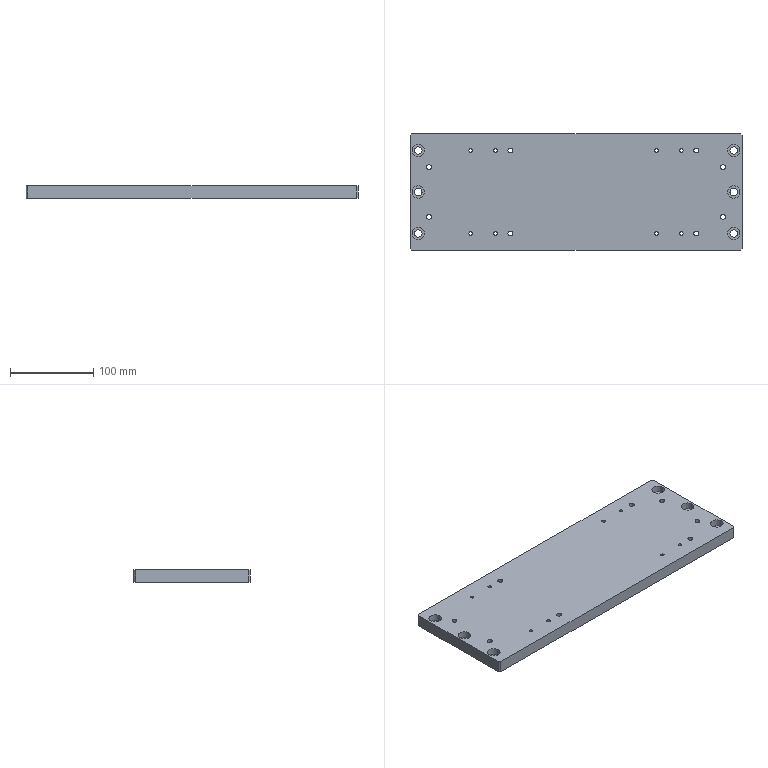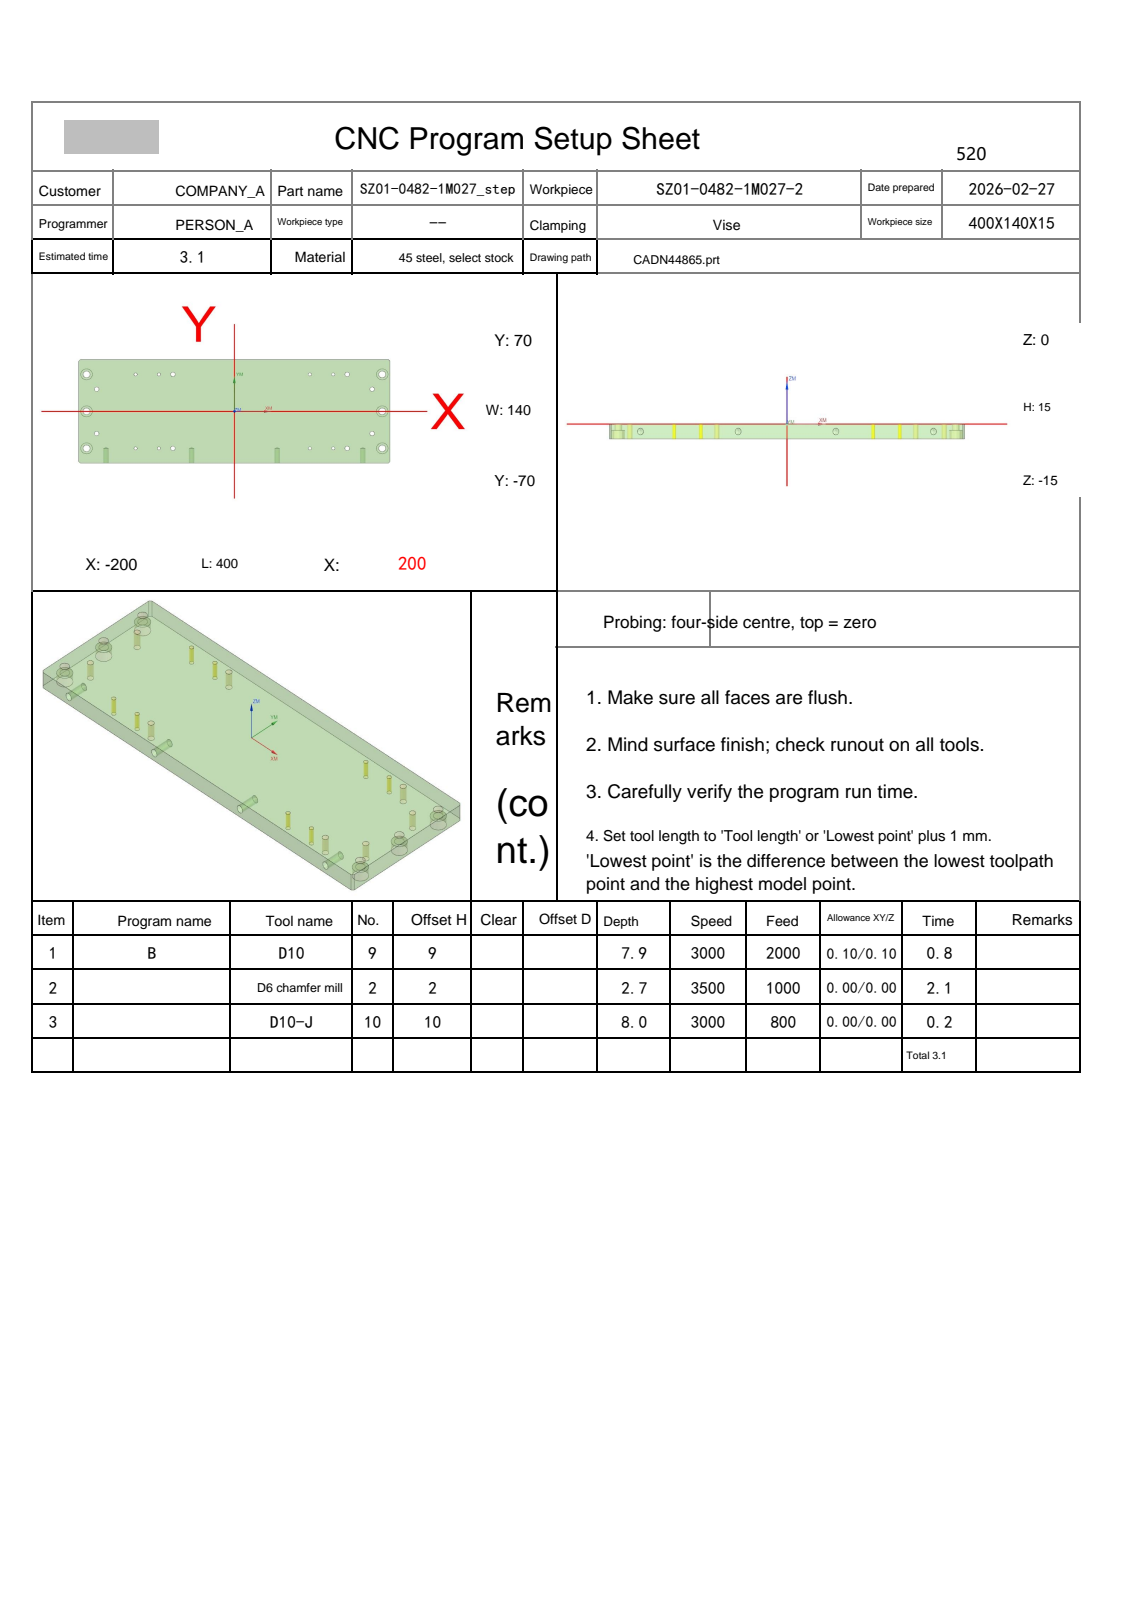NC program | NX | posted by the shop | part box 400 x 140 x 15 mm
Whole program:
%
O0001
(Machine time: 3.63 MIN)
(===Total Tool:3===)
(T9=D10     D=10.  R=0.   D-  H09 Z=-7.9  )
(T2=D6 chamfer mill   D=6.   R=0.   D-  H02 Z=-2.7  )
(T10=D10-J  D=10.  R=0.   D-  H10 Z=-8.   )
G80 G90 G17 G49 G40
G91 G28 Z0
M01
N1 T09 M06
(D10  D=10. R=0. H=09 ce=0.10 di=0.10)
G00 G90 G54 X195.242 Y79.97 M03 S3000
G43 H09 Z50.
M08
Z-.5
G01 X201.606 Y73.606 F2000.
X203.606 Y71.606
X209.97 Y65.242
G00 Z-1.
G01 X203.606 Y71.606
X201.606 Y73.606
X195.242 Y79.97
G00 Z-1.5
G01 X201.606 Y73.606
X203.606 Y71.606
X209.97 Y65.242
G00 Z-2.
G01 X203.606 Y71.606
X201.606 Y73.606
X195.242 Y79.97
G00 Z-2.5
G01 X201.606 Y73.606
X203.606 Y71.606
X209.97 Y65.242
G00 Z-3.
G01 X203.606 Y71.606
X201.606 Y73.606
X195.242 Y79.97
G00 Z-3.5
G01 X201.606 Y73.606
X203.606 Y71.606
X209.97 Y65.242
G00 Z-4.
G01 X203.606 Y71.606
X201.606 Y73.606
X195.242 Y79.97
G00 Z-4.5
G01 X201.606 Y73.606
X203.606 Y71.606
X209.97 Y65.242
G00 Z-5.
G01 X203.606 Y71.606
X201.606 Y73.606
X195.242 Y79.97
G00 Z-5.5
G01 X201.606 Y73.606
X203.606 Y71.606
X209.97 Y65.242
G00 Z-6.
G01 X203.606 Y71.606
X201.606 Y73.606
X195.242 Y79.97
G00 Z-6.5
G01 X201.606 Y73.606
X203.606 Y71.606
X209.97 Y65.242
G00 Z-7.
G01 X203.606 Y71.606
X201.606 Y73.606
X195.242 Y79.97
G00 Z-7.5
G01 X201.606 Y73.606
X203.606 Y71.606
X209.97 Y65.242
G00 Z-7.9
G01 X203.606 Y71.606
X201.606 Y73.606
X195.242 Y79.97
G00 Z50.
X209.97 Y-65.242
Z-.5
G01 X203.606 Y-71.606
X201.606 Y-73.606
X195.242 Y-79.97
G00 Z-1.
G01 X201.606 Y-73.606
X203.606 Y-71.606
X209.97 Y-65.242
G00 Z-1.5
G01 X203.606 Y-71.606
X201.606 Y-73.606
X195.242 Y-79.97
G00 Z-2.
G01 X201.606 Y-73.606
X203.606 Y-71.606
X209.97 Y-65.242
G00 Z-2.5
G01 X203.606 Y-71.606
X201.606 Y-73.606
X195.242 Y-79.97
G00 Z-3.
G01 X201.606 Y-73.606
X203.606 Y-71.606
X209.97 Y-65.242
G00 Z-3.5
G01 X203.606 Y-71.606
X201.606 Y-73.606
X195.242 Y-79.97
G00 Z-4.
G01 X201.606 Y-73.606
X203.606 Y-71.606
X209.97 Y-65.242
G00 Z-4.5
G01 X203.606 Y-71.606
X201.606 Y-73.606
X195.242 Y-79.97
G00 Z-5.
G01 X201.606 Y-73.606
X203.606 Y-71.606
X209.97 Y-65.242
G00 Z-5.5
G01 X203.606 Y-71.606
X201.606 Y-73.606
X195.242 Y-79.97
G00 Z-6.
G01 X201.606 Y-73.606
X203.606 Y-71.606
X209.97 Y-65.242
G00 Z-6.5
G01 X203.606 Y-71.606
X201.606 Y-73.606
X195.242 Y-79.97
G00 Z-7.
G01 X201.606 Y-73.606
X203.606 Y-71.606
X209.97 Y-65.242
G00 Z-7.5
G01 X203.606 Y-71.606
X201.606 Y-73.606
X195.242 Y-79.97
G00 Z-7.9
G01 X201.606 Y-73.606
X203.606 Y-71.606
X209.97 Y-65.242
G00 Z50.
X-195.242 Y-79.97
Z-.5
G01 X-201.606 Y-73.606
X-203.606 Y-71.606
X-209.97 Y-65.242
G00 Z-1.
G01 X-203.606 Y-71.606
X-201.606 Y-73.606
X-195.242 Y-79.97
G00 Z-1.5
G01 X-201.606 Y-73.606
X-203.606 Y-71.606
X-209.97 Y-65.242
G00 Z-2.
G01 X-203.606 Y-71.606
X-201.606 Y-73.606
X-195.242 Y-79.97
G00 Z-2.5
G01 X-201.606 Y-73.606
X-203.606 Y-71.606
X-209.97 Y-65.242
G00 Z-3.
G01 X-203.606 Y-71.606
X-201.606 Y-73.606
X-195.242 Y-79.97
G00 Z-3.5
G01 X-201.606 Y-73.606
X-203.606 Y-71.606
X-209.97 Y-65.242
G00 Z-4.
G01 X-203.606 Y-71.606
X-201.606 Y-73.606
X-195.242 Y-79.97
G00 Z-4.5
G01 X-201.606 Y-73.606
X-203.606 Y-71.606
X-209.97 Y-65.242
G00 Z-5.
G01 X-203.606 Y-71.606
X-201.606 Y-73.606
X-195.242 Y-79.97
G00 Z-5.5
G01 X-201.606 Y-73.606
X-203.606 Y-71.606
X-209.97 Y-65.242
G00 Z-6.
G01 X-203.606 Y-71.606
X-201.606 Y-73.606
X-195.242 Y-79.97
G00 Z-6.5
G01 X-201.606 Y-73.606
X-203.606 Y-71.606
X-209.97 Y-65.242
G00 Z-7.
G01 X-203.606 Y-71.606
X-201.606 Y-73.606
X-195.242 Y-79.97
G00 Z-7.5
G01 X-201.606 Y-73.606
X-203.606 Y-71.606
X-209.97 Y-65.242
G00 Z-7.9
G01 X-203.606 Y-71.606
X-201.606 Y-73.606
X-195.242 Y-79.97
G00 Z50.
X-209.97 Y65.242
Z-.5
G01 X-203.606 Y71.606
X-201.606 Y73.606
X-195.242 Y79.97
G00 Z-1.
G01 X-201.606 Y73.606
X-203.606 Y71.606
X-209.97 Y65.242
G00 Z-1.5
G01 X-203.606 Y71.606
X-201.606 Y73.606
X-195.242 Y79.97
G00 Z-2.
G01 X-201.606 Y73.606
X-203.606 Y71.606
X-209.97 Y65.242
G00 Z-2.5
G01 X-203.606 Y71.606
X-201.606 Y73.606
X-195.242 Y79.97
G00 Z-3.
G01 X-201.606 Y73.606
X-203.606 Y71.606
X-209.97 Y65.242
G00 Z-3.5
G01 X-203.606 Y71.606
X-201.606 Y73.606
X-195.242 Y79.97
G00 Z-4.
G01 X-201.606 Y73.606
X-203.606 Y71.606
X-209.97 Y65.242
G00 Z-4.5
G01 X-203.606 Y71.606
X-201.606 Y73.606
X-195.242 Y79.97
G00 Z-5.
G01 X-201.606 Y73.606
X-203.606 Y71.606
X-209.97 Y65.242
G00 Z-5.5
G01 X-203.606 Y71.606
X-201.606 Y73.606
X-195.242 Y79.97
G00 Z-6.
G01 X-201.606 Y73.606
X-203.606 Y71.606
X-209.97 Y65.242
G00 Z-6.5
G01 X-203.606 Y71.606
X-201.606 Y73.606
X-195.242 Y79.97
G00 Z-7.
G01 X-201.606 Y73.606
X-203.606 Y71.606
X-209.97 Y65.242
G00 Z-7.5
G01 X-203.606 Y71.606
X-201.606 Y73.606
X-195.242 Y79.97
G00 Z-7.9
G01 X-201.606 Y73.606
X-203.606 Y71.606
X-209.97 Y65.242
G00 Z50.
G91 G28 Z0.0
M05
M09
G91 G28 Z0.0
M01
N2 T02 M06
(D6 chamfer mill  D=6. R=0. H=02 ce=0.00 di=0.10)
G00 G90 G54 X97. Y50. M03 S2000
G43 H02 Z50.
M08
G98 G81 X97. Y50. Z-2.7 R3. F100.
X127.
Y-50.
X97.
X-97.
X-127.
Y50.
X-97.
G80
G00 Z50.
G00 G90 X-.386 Y71.227 M03 S3500
Z50.
Z.172
G01 Z-1.2 F1000.
G03 X-.1 Y71.027 I1.286 J1.532
G01 X-.054 Y70.997
X0.0 Y71.
X198.
X198.259 Y70.966
X198.5 Y70.866
X198.707 Y70.707
X200.707 Y68.707
X200.866 Y68.5
X200.966 Y68.259
X201. Y68.
Y-68.
X200.966 Y-68.259
X200.866 Y-68.5
X200.707 Y-68.707
X198.707 Y-70.707
X198.5 Y-70.866
X198.259 Y-70.966
X198. Y-71.
X-198.
X-198.259 Y-70.966
X-198.5 Y-70.866
X-198.707 Y-70.707
X-200.707 Y-68.707
X-200.866 Y-68.5
X-200.966 Y-68.259
X-201. Y-68.
Y68.
X-200.966 Y68.259
X-200.866 Y68.5
X-200.707 Y68.707
X-198.707 Y70.707
X-198.5 Y70.866
X-198.259 Y70.966
X-198. Y71.
X0.0
X.054 Y70.997
X.1 Y71.027
G03 X.386 Y71.227 I-1. J1.732
G01 Z.172
G00 Z10.
X186.697 Y-49.599
Z.23
G01 Z-1.2
G03 X186.519 Y-49.898 I1.624 J-1.167
G01 X186.493 Y-49.946
X186.5 Y-50.
G03 X190. Y-53.5 I3.5 J0.0
X193.5 Y-50. I0.0 J3.5
X190. Y-46.5 I-3.5 J0.0
X186.5 Y-50. I0.0 J-3.5
G01 X186.493 Y-50.054
X186.519 Y-50.102
G03 X186.697 Y-50.401 I1.802 J.868
G01 Z.23
G00 Z10.
X143.192 Y-49.596
Z.257
G01 Z-1.2
G03 X143.018 Y-49.898 I1.638 J-1.147
G01 X142.992 Y-49.946
X143. Y-50.
G03 X145. Y-52. I2. J0.0
X147. Y-50. I0.0 J2.
X145. Y-48. I-2. J0.0
X143.03 Y-49.653 I0.0 J-2.
G01 X143. Y-50.
X142.992 Y-50.054
X143.018 Y-50.102
G03 X143.192 Y-50.404 I1.813 J.845
G01 Z.257
G00 Z10.
X126.074 Y-49.588
Z.32
G01 Z-1.2
G03 X125.914 Y-49.897 I1.687 J-1.075
G01 X125.89 Y-49.946
X125.9 Y-50.
G03 X127. Y-51.1 I1.1 J0.0
X128.1 Y-50. I0.0 J1.1
X127. Y-48.9 I-1.1 J0.0
X125.9 Y-50. I0.0 J-1.1
G01 X125.89 Y-50.054
X125.914 Y-50.103
G03 X126.074 Y-50.412 I1.848 J.765
G01 Z.32
G00 Z10.
X96.074 Y-49.588
Z.32
G01 Z-1.2
G03 X95.914 Y-49.897 I1.687 J-1.075
G01 X95.89 Y-49.946
X95.9 Y-50.
G03 X97. Y-51.1 I1.1 J0.0
X98.1 Y-50. I0.0 J1.1
X97. Y-48.9 I-1.1 J0.0
X95.9 Y-50. I0.0 J-1.1
G01 X95.89 Y-50.054
X95.914 Y-50.103
G03 X96.074 Y-50.412 I1.848 J.765
G01 Z.32
G00 Z10.
X175.192 Y-29.596
Z.257
G01 Z-1.2
G03 X175.018 Y-29.898 I1.638 J-1.147
G01 X174.992 Y-29.946
X175. Y-30.
G03 X177. Y-32. I2. J0.0
X179. Y-30. I0.0 J2.
X177. Y-28. I-2. J0.0
X175.03 Y-29.653 I0.0 J-2.
G01 X175. Y-30.
X174.992 Y-30.054
X175.018 Y-30.102
G03 X175.192 Y-30.404 I1.813 J.845
G01 Z.257
G00 Z10.
X186.697 Y.401
Z.23
G01 Z-1.2
G03 X186.519 Y.102 I1.624 J-1.167
G01 X186.493 Y.054
X186.5 Y0.0
G03 X190. Y-3.5 I3.5 J0.0
X193.5 Y0.0 I0.0 J3.5
X190. Y3.5 I-3.5 J0.0
X186.5 Y0.0 I0.0 J-3.5
G01 X186.493 Y-.054
X186.519 Y-.102
G03 X186.697 Y-.401 I1.802 J.868
G01 Z.23
G00 Z10.
X175.192 Y30.404
Z.257
G01 Z-1.2
G03 X175.018 Y30.102 I1.638 J-1.147
G01 X174.992 Y30.054
X175. Y30.
G03 X177. Y28. I2. J0.0
X179. Y30. I0.0 J2.
X177. Y32. I-2. J0.0
X175.03 Y30.347 I0.0 J-2.
G01 X175. Y30.
X174.992 Y29.946
X175.018 Y29.898
G03 X175.192 Y29.596 I1.813 J.845
G01 Z.257
G00 Z10.
X186.697 Y50.401
Z.23
G01 Z-1.2
G03 X186.519 Y50.102 I1.624 J-1.167
G01 X186.493 Y50.054
X186.5 Y50.
G03 X190. Y46.5 I3.5 J0.0
X193.5 Y50. I0.0 J3.5
X190. Y53.5 I-3.5 J0.0
X186.5 Y50. I0.0 J-3.5
G01 X186.493 Y49.946
X186.519 Y49.898
G03 X186.697 Y49.599 I1.802 J.868
G01 Z.23
G00 Z10.
X143.192 Y50.404
Z.257
G01 Z-1.2
G03 X143.018 Y50.102 I1.638 J-1.147
G01 X142.992 Y50.054
X143. Y50.
G03 X145. Y48. I2. J0.0
X147. Y50. I0.0 J2.
X145. Y52. I-2. J0.0
X143.03 Y50.347 I0.0 J-2.
G01 X143. Y50.
X142.992 Y49.946
X143.018 Y49.898
G03 X143.192 Y49.596 I1.813 J.845
G01 Z.257
G00 Z10.
X126.074 Y50.412
Z.32
G01 Z-1.2
G03 X125.914 Y50.103 I1.687 J-1.075
G01 X125.89 Y50.054
X125.9 Y50.
G03 X127. Y48.9 I1.1 J0.0
X128.1 Y50. I0.0 J1.1
X127. Y51.1 I-1.1 J0.0
X125.9 Y50. I0.0 J-1.1
G01 X125.89 Y49.946
X125.914 Y49.897
G03 X126.074 Y49.588 I1.848 J.765
G01 Z.32
G00 Z10.
X96.074 Y50.412
Z.32
G01 Z-1.2
G03 X95.914 Y50.103 I1.687 J-1.075
G01 X95.89 Y50.054
X95.9 Y50.
G03 X97. Y48.9 I1.1 J0.0
X98.1 Y50. I0.0 J1.1
X97. Y51.1 I-1.1 J0.0
X95.9 Y50. I0.0 J-1.1
G01 X95.89 Y49.946
X95.914 Y49.897
G03 X96.074 Y49.588 I1.848 J.765
G01 Z.32
G00 Z10.
X-80.808 Y50.404
Z.257
G01 Z-1.2
G03 X-80.982 Y50.102 I1.638 J-1.147
G01 X-81.008 Y50.054
X-81. Y50.
G03 X-79. Y48. I2. J0.0
X-77. Y50. I0.0 J2.
X-79. Y52. I-2. J0.0
X-80.97 Y50.347 I0.0 J-2.
G01 X-81. Y50.
X-81.008 Y49.946
X-80.982 Y49.898
G03 X-80.808 Y49.596 I1.813 J.845
G01 Z.257
G00 Z10.
X-97.926 Y50.412
Z.32
G01 Z-1.2
G03 X-98.086 Y50.103 I1.687 J-1.075
G01 X-98.11 Y50.054
X-98.1 Y50.
G03 X-97. Y48.9 I1.1 J0.0
X-95.9 Y50. I0.0 J1.1
X-97. Y51.1 I-1.1 J0.0
X-98.1 Y50. I0.0 J-1.1
G01 X-98.11 Y49.946
X-98.086 Y49.897
G03 X-97.926 Y49.588 I1.848 J.765
G01 Z.32
G00 Z10.
X-127.926 Y50.412
Z.32
G01 Z-1.2
G03 X-128.086 Y50.103 I1.687 J-1.075
G01 X-128.11 Y50.054
X-128.1 Y50.
G03 X-127. Y48.9 I1.1 J0.0
X-125.9 Y50. I0.0 J1.1
X-127. Y51.1 I-1.1 J0.0
X-128.1 Y50. I0.0 J-1.1
G01 X-128.11 Y49.946
X-128.086 Y49.897
G03 X-127.926 Y49.588 I1.848 J.765
G01 Z.32
G00 Z10.
X-193.303 Y50.401
Z.23
G01 Z-1.2
G03 X-193.481 Y50.102 I1.624 J-1.167
G01 X-193.507 Y50.054
X-193.5 Y50.
G03 X-190. Y46.5 I3.5 J0.0
X-186.5 Y50. I0.0 J3.5
X-190. Y53.5 I-3.5 J0.0
X-193.5 Y50. I0.0 J-3.5
G01 X-193.507 Y49.946
X-193.481 Y49.898
G03 X-193.303 Y49.599 I1.802 J.868
G01 Z.23
G00 Z10.
X-178.808 Y30.404
Z.257
G01 Z-1.2
G03 X-178.982 Y30.102 I1.638 J-1.147
G01 X-179.008 Y30.054
X-179. Y30.
G03 X-177. Y28. I2. J0.0
X-175. Y30. I0.0 J2.
X-177. Y32. I-2. J0.0
X-178.97 Y30.347 I0.0 J-2.
G01 X-179. Y30.
X-179.008 Y29.946
X-178.982 Y29.898
G03 X-178.808 Y29.596 I1.813 J.845
G01 Z.257
G00 Z10.
X-193.303 Y.401
Z.23
G01 Z-1.2
G03 X-193.481 Y.102 I1.624 J-1.167
G01 X-193.507 Y.054
X-193.5 Y0.0
G03 X-190. Y-3.5 I3.5 J0.0
X-186.5 Y0.0 I0.0 J3.5
X-190. Y3.5 I-3.5 J0.0
X-193.5 Y0.0 I0.0 J-3.5
G01 X-193.507 Y-.054
X-193.481 Y-.102
G03 X-193.303 Y-.401 I1.802 J.868
G01 Z.23
G00 Z10.
X-178.808 Y-29.596
Z.257
G01 Z-1.2
G03 X-178.982 Y-29.898 I1.638 J-1.147
G01 X-179.008 Y-29.946
X-179. Y-30.
G03 X-177. Y-32. I2. J0.0
X-175. Y-30. I0.0 J2.
X-177. Y-28. I-2. J0.0
X-178.97 Y-29.653 I0.0 J-2.
G01 X-179. Y-30.
X-179.008 Y-30.054
X-178.982 Y-30.102
G03 X-178.808 Y-30.404 I1.813 J.845
G01 Z.257
G00 Z10.
X-193.303 Y-49.599
Z.23
G01 Z-1.2
G03 X-193.481 Y-49.898 I1.624 J-1.167
G01 X-193.507 Y-49.946
X-193.5 Y-50.
G03 X-190. Y-53.5 I3.5 J0.0
X-186.5 Y-50. I0.0 J3.5
X-190. Y-46.5 I-3.5 J0.0
X-193.5 Y-50. I0.0 J-3.5
G01 X-193.507 Y-50.054
X-193.481 Y-50.102
G03 X-193.303 Y-50.401 I1.802 J.868
G01 Z.23
G00 Z10.
X-127.926 Y-49.588
Z.32
G01 Z-1.2
G03 X-128.086 Y-49.897 I1.687 J-1.075
G01 X-128.11 Y-49.946
X-128.1 Y-50.
G03 X-127. Y-51.1 I1.1 J0.0
X-125.9 Y-50. I0.0 J1.1
X-127. Y-48.9 I-1.1 J0.0
X-128.1 Y-50. I0.0 J-1.1
G01 X-128.11 Y-50.054
X-128.086 Y-50.103
G03 X-127.926 Y-50.412 I1.848 J.765
G01 Z.32
G00 Z10.
X-97.926 Y-49.588
Z.32
G01 Z-1.2
G03 X-98.086 Y-49.897 I1.687 J-1.075
G01 X-98.11 Y-49.946
X-98.1 Y-50.
G03 X-97. Y-51.1 I1.1 J0.0
X-95.9 Y-50. I0.0 J1.1
X-97. Y-48.9 I-1.1 J0.0
X-98.1 Y-50. I0.0 J-1.1
G01 X-98.11 Y-50.054
X-98.086 Y-50.103
G03 X-97.926 Y-50.412 I1.848 J.765
G01 Z.32
G00 Z10.
X-80.808 Y-49.596
Z.257
G01 Z-1.2
G03 X-80.982 Y-49.898 I1.638 J-1.147
G01 X-81.008 Y-49.946
X-81. Y-50.
G03 X-79. Y-52. I2. J0.0
X-77. Y-50. I0.0 J2.
X-79. Y-48. I-2. J0.0
X-80.97 Y-49.653 I0.0 J-2.
G01 X-81. Y-50.
X-81.008 Y-50.054
X-80.982 Y-50.102
G03 X-80.808 Y-50.404 I1.813 J.845
G01 Z.257
G00 Z50.
G91 G28 Z0.0
M05
M09
G91 G28 Z0.0
M01
N3 T10 M06
(D10-J  D=10. R=0. H=10 ce=0.00 di=0.00)
G00 G90 G54 X197.293 Y77.778 M03 S3000
G43 H10 Z50.
M08
Z-7.
G01 Z-8. F800.
X201.536 Y73.536
X203.536 Y71.536
X207.778 Y67.293
Z-7.
G00 Z50.
Y-67.293
Z-7.
G01 Z-8.
X203.536 Y-71.536
X201.536 Y-73.536
X197.293 Y-77.778
Z-7.
G00 Z50.
X-197.293
Z-7.
G01 Z-8.
X-201.536 Y-73.536
X-203.536 Y-71.536
X-207.778 Y-67.293
Z-7.
G00 Z50.
Y67.293
Z-7.
G01 Z-8.
X-203.536 Y71.536
X-201.536 Y73.536
X-197.293 Y77.778
Z-7.
G00 Z50.
M05
M09
G91 G28 Z0.0
G91 G28 Y0.0
M30
%